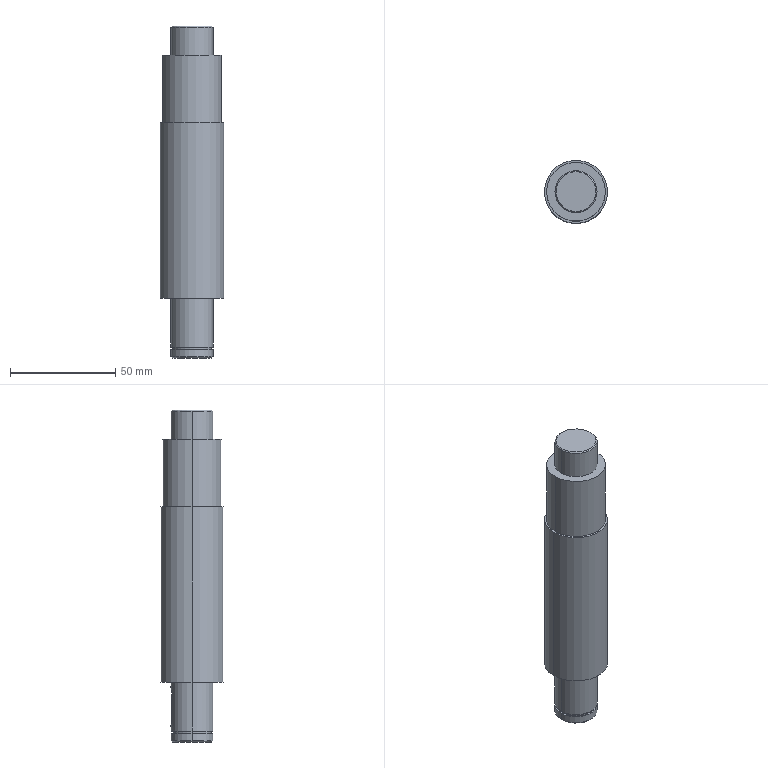Part | SolidWorks | features BaseBody 1 | 1 solid | 28 faces | box 30 x 30 x 157.8 mm | volume 91673 mm3 | cylinder 14 | plane 10 | cone 4 | commonest cylinder face diameters 20 x6 6 x2 18.35 x2 28 x2 30 x2
STEP:
#1=CARTESIAN_POINT('',(9.175,0.,5.2));
#2=VERTEX_POINT('',#1);
#3=CARTESIAN_POINT('',(-9.175,0.,5.2));
#4=VERTEX_POINT('',#3);
#5=CARTESIAN_POINT('',(0.,0.,5.2));
#6=DIRECTION('',(0.,0.,1.));
#7=DIRECTION('',(1.,0.,0.));
#8=AXIS2_PLACEMENT_3D('',#5,#6,#7);
#9=CIRCLE('',#8,9.175);
#10=EDGE_CURVE('',#2,#4,#9,.T.);
#11=ORIENTED_EDGE('',*,*,#10,.F.);
#12=CARTESIAN_POINT('',(9.175,0.,4.));
#13=VERTEX_POINT('',#12);
#14=CARTESIAN_POINT('',(9.175,0.,4.6));
#15=DIRECTION('',(0.,0.,-1.));
#16=VECTOR('',#15,1000.);
#17=LINE('',#14,#16);
#18=EDGE_CURVE('',#2,#13,#17,.T.);
#19=ORIENTED_EDGE('',*,*,#18,.T.);
#20=CARTESIAN_POINT('',(-9.175,0.,4.));
#21=VERTEX_POINT('',#20);
#22=CARTESIAN_POINT('',(0.,0.,4.));
#23=DIRECTION('',(0.,0.,1.));
#24=DIRECTION('',(1.,0.,0.));
#25=AXIS2_PLACEMENT_3D('',#22,#23,#24);
#26=CIRCLE('',#25,9.175);
#27=EDGE_CURVE('',#13,#21,#26,.T.);
#28=ORIENTED_EDGE('',*,*,#27,.T.);
#29=CARTESIAN_POINT('',(-9.175,0.,4.6));
#30=DIRECTION('',(0.,0.,-1.));
#31=VECTOR('',#30,1000.);
#32=LINE('',#29,#31);
#33=EDGE_CURVE('',#4,#21,#32,.T.);
#34=ORIENTED_EDGE('',*,*,#33,.F.);
#35=EDGE_LOOP('',(#11,#19,#28,#34));
#36=FACE_OUTER_BOUND('',#35,.T.);
#37=CARTESIAN_POINT('',(0.,0.,4.6));
#38=DIRECTION('',(0.,0.,-1.));
#39=DIRECTION('',(-1.,0.,0.));
#40=AXIS2_PLACEMENT_3D('',#37,#38,#39);
#41=CYLINDRICAL_SURFACE('',#40,9.175);
#42=ADVANCED_FACE('',(#36),#41,.T.);
#43=CARTESIAN_POINT('',(3.,9.539,10.789));
#44=VERTEX_POINT('',#43);
#45=CARTESIAN_POINT('',(3.,9.539,22.789));
#46=VERTEX_POINT('',#45);
#47=CARTESIAN_POINT('',(3.,9.539,0.));
#48=DIRECTION('',(0.,0.,1.));
#49=VECTOR('',#48,1000.);
#50=LINE('',#47,#49);
#51=EDGE_CURVE('',#44,#46,#50,.T.);
#52=ORIENTED_EDGE('',*,*,#51,.T.);
#53=CARTESIAN_POINT('',(-3.,9.539,22.789));
#54=VERTEX_POINT('',#53);
#55=CARTESIAN_POINT('',(3.,9.539,22.789));
#56=CARTESIAN_POINT('',(3.,9.539,22.988));
#57=CARTESIAN_POINT('',(2.98,9.546,23.184));
#58=CARTESIAN_POINT('',(2.904,9.569,23.569));
#59=CARTESIAN_POINT('',(2.845,9.587,23.76));
#60=CARTESIAN_POINT('',(2.695,9.63,24.122));
#61=CARTESIAN_POINT('',(2.602,9.656,24.294));
#62=CARTESIAN_POINT('',(2.385,9.712,24.619));
#63=CARTESIAN_POINT('',(2.259,9.742,24.772));
#64=CARTESIAN_POINT('',(1.847,9.832,25.185));
#65=CARTESIAN_POINT('',(1.515,9.891,25.408));
#66=CARTESIAN_POINT('',(0.9743,9.954,25.633));
#67=CARTESIAN_POINT('',(0.7844,9.971,25.691));
#68=CARTESIAN_POINT('',(0.396,9.994,25.769));
#69=CARTESIAN_POINT('',(0.1993,10.,25.789));
#70=CARTESIAN_POINT('',(-0.1994,10.,25.789));
#71=CARTESIAN_POINT('',(-0.3951,9.994,25.769));
#72=CARTESIAN_POINT('',(-0.7799,9.971,25.692));
#73=CARTESIAN_POINT('',(-0.971,9.954,25.634));
#74=CARTESIAN_POINT('',(-1.334,9.912,25.483));
#75=CARTESIAN_POINT('',(-1.505,9.887,25.391));
#76=CARTESIAN_POINT('',(-1.831,9.832,25.174));
#77=CARTESIAN_POINT('',(-1.984,9.802,25.048));
#78=CARTESIAN_POINT('',(-2.396,9.713,24.636));
#79=CARTESIAN_POINT('',(-2.619,9.652,24.303));
#80=CARTESIAN_POINT('',(-2.844,9.587,23.763));
#81=CARTESIAN_POINT('',(-2.902,9.57,23.573));
#82=CARTESIAN_POINT('',(-2.98,9.546,23.185));
#83=CARTESIAN_POINT('',(-3.,9.539,22.988));
#84=CARTESIAN_POINT('',(-3.,9.539,22.789));
#85=B_SPLINE_CURVE_WITH_KNOTS('',3,(#55,#56,#57,#58,#59,#60,#61,#62,#63,#64,#65,#66,#67,#68,#69,#70,#71,#72,#73,#74,#75,#76,#77,#78,#79,#80,#81,#82,#83,#84),.UNSPECIFIED.,.F.,.F.,(4,2,2,2,2,2,2,2,2,2,2,2,2,2,4),(0.,0.0005892,0.001178,0.001768,0.002357,0.003535,0.004125,0.004714,0.005303,0.005892,0.006482,0.007071,0.008249,0.008838,0.009428),.UNSPECIFIED.);
#86=EDGE_CURVE('',#46,#54,#85,.T.);
#87=ORIENTED_EDGE('',*,*,#86,.T.);
#88=CARTESIAN_POINT('',(-3.,9.539,10.789));
#89=VERTEX_POINT('',#88);
#90=CARTESIAN_POINT('',(-3.,9.539,0.));
#91=DIRECTION('',(0.,0.,-1.));
#92=VECTOR('',#91,1000.);
#93=LINE('',#90,#92);
#94=EDGE_CURVE('',#54,#89,#93,.T.);
#95=ORIENTED_EDGE('',*,*,#94,.T.);
#96=CARTESIAN_POINT('',(-3.,9.539,10.789));
#97=CARTESIAN_POINT('',(-3.,9.539,10.59));
#98=CARTESIAN_POINT('',(-2.98,9.546,10.394));
#99=CARTESIAN_POINT('',(-2.904,9.569,10.009));
#100=CARTESIAN_POINT('',(-2.845,9.587,9.818));
#101=CARTESIAN_POINT('',(-2.695,9.63,9.456));
#102=CARTESIAN_POINT('',(-2.602,9.656,9.284));
#103=CARTESIAN_POINT('',(-2.385,9.712,8.959));
#104=CARTESIAN_POINT('',(-2.259,9.742,8.806));
#105=CARTESIAN_POINT('',(-1.847,9.832,8.393));
#106=CARTESIAN_POINT('',(-1.515,9.891,8.17));
#107=CARTESIAN_POINT('',(-0.9743,9.954,7.945));
#108=CARTESIAN_POINT('',(-0.7844,9.971,7.887));
#109=CARTESIAN_POINT('',(-0.396,9.994,7.809));
#110=CARTESIAN_POINT('',(-0.1993,10.,7.789));
#111=CARTESIAN_POINT('',(0.1994,10.,7.789));
#112=CARTESIAN_POINT('',(0.3951,9.994,7.809));
#113=CARTESIAN_POINT('',(0.7799,9.971,7.886));
#114=CARTESIAN_POINT('',(0.971,9.954,7.944));
#115=CARTESIAN_POINT('',(1.334,9.912,8.095));
#116=CARTESIAN_POINT('',(1.505,9.887,8.187));
#117=CARTESIAN_POINT('',(1.831,9.832,8.404));
#118=CARTESIAN_POINT('',(1.984,9.802,8.53));
#119=CARTESIAN_POINT('',(2.396,9.713,8.942));
#120=CARTESIAN_POINT('',(2.619,9.652,9.275));
#121=CARTESIAN_POINT('',(2.844,9.587,9.815));
#122=CARTESIAN_POINT('',(2.902,9.57,10.005));
#123=CARTESIAN_POINT('',(2.98,9.546,10.393));
#124=CARTESIAN_POINT('',(3.,9.539,10.59));
#125=CARTESIAN_POINT('',(3.,9.539,10.789));
#126=B_SPLINE_CURVE_WITH_KNOTS('',3,(#96,#97,#98,#99,#100,#101,#102,#103,#104,#105,#106,#107,#108,#109,#110,#111,#112,#113,#114,#115,#116,#117,#118,#119,#120,#121,#122,#123,#124,#125),.UNSPECIFIED.,.F.,.F.,(4,2,2,2,2,2,2,2,2,2,2,2,2,2,4),(0.,0.0005892,0.001178,0.001768,0.002357,0.003535,0.004125,0.004714,0.005303,0.005892,0.006482,0.007071,0.008249,0.008838,0.009428),.UNSPECIFIED.);
#127=EDGE_CURVE('',#89,#44,#126,.T.);
#128=ORIENTED_EDGE('',*,*,#127,.T.);
#129=EDGE_LOOP('',(#52,#87,#95,#128));
#130=FACE_BOUND('',#129,.T.);
#131=CARTESIAN_POINT('',(10.,0.,28.378));
#132=VERTEX_POINT('',#131);
#133=CARTESIAN_POINT('',(-10.,0.,28.378));
#134=VERTEX_POINT('',#133);
#135=CARTESIAN_POINT('',(0.,0.,28.378));
#136=DIRECTION('',(0.,0.,1.));
#137=DIRECTION('',(-1.,0.,0.));
#138=AXIS2_PLACEMENT_3D('',#135,#136,#137);
#139=CIRCLE('',#138,10.);
#140=EDGE_CURVE('',#132,#134,#139,.T.);
#141=ORIENTED_EDGE('',*,*,#140,.F.);
#142=CARTESIAN_POINT('',(10.,0.,5.2));
#143=VERTEX_POINT('',#142);
#144=CARTESIAN_POINT('',(10.,0.,0.));
#145=DIRECTION('',(0.,0.,-1.));
#146=VECTOR('',#145,1000.);
#147=LINE('',#144,#146);
#148=EDGE_CURVE('',#132,#143,#147,.T.);
#149=ORIENTED_EDGE('',*,*,#148,.T.);
#150=CARTESIAN_POINT('',(-10.,0.,5.2));
#151=VERTEX_POINT('',#150);
#152=CARTESIAN_POINT('',(0.,0.,5.2));
#153=DIRECTION('',(0.,0.,1.));
#154=DIRECTION('',(-1.,0.,0.));
#155=AXIS2_PLACEMENT_3D('',#152,#153,#154);
#156=CIRCLE('',#155,10.);
#157=EDGE_CURVE('',#143,#151,#156,.T.);
#158=ORIENTED_EDGE('',*,*,#157,.T.);
#159=CARTESIAN_POINT('',(-10.,0.,0.));
#160=DIRECTION('',(0.,0.,-1.));
#161=VECTOR('',#160,1000.);
#162=LINE('',#159,#161);
#163=EDGE_CURVE('',#134,#151,#162,.T.);
#164=ORIENTED_EDGE('',*,*,#163,.F.);
#165=EDGE_LOOP('',(#141,#149,#158,#164));
#166=FACE_OUTER_BOUND('',#165,.T.);
#167=CARTESIAN_POINT('',(0.,0.,0.));
#168=DIRECTION('',(0.,0.,-1.));
#169=DIRECTION('',(-1.,0.,0.));
#170=AXIS2_PLACEMENT_3D('',#167,#168,#169);
#171=CYLINDRICAL_SURFACE('',#170,10.);
#172=ADVANCED_FACE('',(#130,#166),#171,.T.);
#173=CARTESIAN_POINT('',(-9.5,0.,157.8));
#174=VERTEX_POINT('',#173);
#175=CARTESIAN_POINT('',(9.5,0.,157.8));
#176=VERTEX_POINT('',#175);
#177=CARTESIAN_POINT('',(0.,0.,157.8));
#178=DIRECTION('',(0.,0.,-1.));
#179=DIRECTION('',(-1.,0.,0.));
#180=AXIS2_PLACEMENT_3D('',#177,#178,#179);
#181=CIRCLE('',#180,9.5);
#182=EDGE_CURVE('',#174,#176,#181,.T.);
#183=ORIENTED_EDGE('',*,*,#182,.T.);
#184=CARTESIAN_POINT('',(10.,0.,157.3));
#185=VERTEX_POINT('',#184);
#186=CARTESIAN_POINT('',(9.75,0.,157.55));
#187=DIRECTION('',(0.7071,0.,-0.7071));
#188=VECTOR('',#187,1000.);
#189=LINE('',#186,#188);
#190=EDGE_CURVE('',#176,#185,#189,.T.);
#191=ORIENTED_EDGE('',*,*,#190,.T.);
#192=CARTESIAN_POINT('',(-10.,0.,157.3));
#193=VERTEX_POINT('',#192);
#194=CARTESIAN_POINT('',(0.,0.,157.3));
#195=DIRECTION('',(0.,0.,1.));
#196=DIRECTION('',(-1.,0.,0.));
#197=AXIS2_PLACEMENT_3D('',#194,#195,#196);
#198=CIRCLE('',#197,10.);
#199=EDGE_CURVE('',#185,#193,#198,.T.);
#200=ORIENTED_EDGE('',*,*,#199,.T.);
#201=CARTESIAN_POINT('',(-9.75,0.,157.55));
#202=DIRECTION('',(-0.7071,0.,-0.7071));
#203=VECTOR('',#202,1000.);
#204=LINE('',#201,#203);
#205=EDGE_CURVE('',#174,#193,#204,.T.);
#206=ORIENTED_EDGE('',*,*,#205,.F.);
#207=EDGE_LOOP('',(#183,#191,#200,#206));
#208=FACE_OUTER_BOUND('',#207,.T.);
#209=CARTESIAN_POINT('',(0.,0.,157.55));
#210=DIRECTION('',(0.,0.,-1.));
#211=DIRECTION('',(-1.,0.,0.));
#212=AXIS2_PLACEMENT_3D('',#209,#210,#211);
#213=CONICAL_SURFACE('',#212,9.75,0.7854);
#214=ADVANCED_FACE('',(#208),#213,.T.);
#215=ORIENTED_EDGE('',*,*,#199,.F.);
#216=CARTESIAN_POINT('',(10.,0.,143.8));
#217=VERTEX_POINT('',#216);
#218=CARTESIAN_POINT('',(10.,0.,143.8));
#219=DIRECTION('',(0.,0.,-1.));
#220=VECTOR('',#219,1000.);
#221=LINE('',#218,#220);
#222=EDGE_CURVE('',#185,#217,#221,.T.);
#223=ORIENTED_EDGE('',*,*,#222,.T.);
#224=CARTESIAN_POINT('',(-10.,0.,143.8));
#225=VERTEX_POINT('',#224);
#226=CARTESIAN_POINT('',(0.,0.,143.8));
#227=DIRECTION('',(0.,0.,-1.));
#228=DIRECTION('',(-1.,0.,0.));
#229=AXIS2_PLACEMENT_3D('',#226,#227,#228);
#230=CIRCLE('',#229,10.);
#231=EDGE_CURVE('',#225,#217,#230,.T.);
#232=ORIENTED_EDGE('',*,*,#231,.F.);
#233=CARTESIAN_POINT('',(-10.,0.,143.8));
#234=DIRECTION('',(0.,0.,-1.));
#235=VECTOR('',#234,1000.);
#236=LINE('',#233,#235);
#237=EDGE_CURVE('',#193,#225,#236,.T.);
#238=ORIENTED_EDGE('',*,*,#237,.F.);
#239=EDGE_LOOP('',(#215,#223,#232,#238));
#240=FACE_OUTER_BOUND('',#239,.T.);
#241=CARTESIAN_POINT('',(0.,0.,143.8));
#242=DIRECTION('',(0.,0.,-1.));
#243=DIRECTION('',(-1.,0.,0.));
#244=AXIS2_PLACEMENT_3D('',#241,#242,#243);
#245=CYLINDRICAL_SURFACE('',#244,10.);
#246=ADVANCED_FACE('',(#240),#245,.T.);
#247=CARTESIAN_POINT('',(-9.5,0.,0.));
#248=VERTEX_POINT('',#247);
#249=CARTESIAN_POINT('',(9.5,0.,0.));
#250=VERTEX_POINT('',#249);
#251=CARTESIAN_POINT('',(0.,0.,0.));
#252=DIRECTION('',(0.,0.,1.));
#253=DIRECTION('',(-1.,0.,0.));
#254=AXIS2_PLACEMENT_3D('',#251,#252,#253);
#255=CIRCLE('',#254,9.5);
#256=EDGE_CURVE('',#248,#250,#255,.T.);
#257=ORIENTED_EDGE('',*,*,#256,.T.);
#258=CARTESIAN_POINT('',(10.,0.,0.5));
#259=VERTEX_POINT('',#258);
#260=CARTESIAN_POINT('',(9.75,0.,0.25));
#261=DIRECTION('',(0.7071,0.,0.7071));
#262=VECTOR('',#261,1000.);
#263=LINE('',#260,#262);
#264=EDGE_CURVE('',#250,#259,#263,.T.);
#265=ORIENTED_EDGE('',*,*,#264,.T.);
#266=CARTESIAN_POINT('',(-10.,0.,0.5));
#267=VERTEX_POINT('',#266);
#268=CARTESIAN_POINT('',(0.,0.,0.5));
#269=DIRECTION('',(0.,0.,-1.));
#270=DIRECTION('',(-1.,0.,0.));
#271=AXIS2_PLACEMENT_3D('',#268,#269,#270);
#272=CIRCLE('',#271,10.);
#273=EDGE_CURVE('',#259,#267,#272,.T.);
#274=ORIENTED_EDGE('',*,*,#273,.T.);
#275=CARTESIAN_POINT('',(-9.75,0.,0.25));
#276=DIRECTION('',(-0.7071,0.,0.7071));
#277=VECTOR('',#276,1000.);
#278=LINE('',#275,#277);
#279=EDGE_CURVE('',#248,#267,#278,.T.);
#280=ORIENTED_EDGE('',*,*,#279,.F.);
#281=EDGE_LOOP('',(#257,#265,#274,#280));
#282=FACE_OUTER_BOUND('',#281,.T.);
#283=CARTESIAN_POINT('',(0.,0.,0.25));
#284=DIRECTION('',(0.,0.,1.));
#285=DIRECTION('',(-1.,0.,0.));
#286=AXIS2_PLACEMENT_3D('',#283,#284,#285);
#287=CONICAL_SURFACE('',#286,9.75,0.7854);
#288=ADVANCED_FACE('',(#282),#287,.T.);
#289=CARTESIAN_POINT('',(-10.,0.,4.));
#290=VERTEX_POINT('',#289);
#291=CARTESIAN_POINT('',(10.,0.,4.));
#292=VERTEX_POINT('',#291);
#293=CARTESIAN_POINT('',(0.,0.,4.));
#294=DIRECTION('',(0.,0.,-1.));
#295=DIRECTION('',(-1.,0.,0.));
#296=AXIS2_PLACEMENT_3D('',#293,#294,#295);
#297=CIRCLE('',#296,10.);
#298=EDGE_CURVE('',#290,#292,#297,.T.);
#299=ORIENTED_EDGE('',*,*,#298,.T.);
#300=CARTESIAN_POINT('',(10.,0.,0.));
#301=DIRECTION('',(0.,0.,-1.));
#302=VECTOR('',#301,1000.);
#303=LINE('',#300,#302);
#304=EDGE_CURVE('',#292,#259,#303,.T.);
#305=ORIENTED_EDGE('',*,*,#304,.T.);
#306=CARTESIAN_POINT('',(0.,0.,0.5));
#307=DIRECTION('',(0.,0.,-1.));
#308=DIRECTION('',(-1.,0.,0.));
#309=AXIS2_PLACEMENT_3D('',#306,#307,#308);
#310=CIRCLE('',#309,10.);
#311=EDGE_CURVE('',#267,#259,#310,.T.);
#312=ORIENTED_EDGE('',*,*,#311,.F.);
#313=CARTESIAN_POINT('',(-10.,0.,0.));
#314=DIRECTION('',(0.,0.,-1.));
#315=VECTOR('',#314,1000.);
#316=LINE('',#313,#315);
#317=EDGE_CURVE('',#290,#267,#316,.T.);
#318=ORIENTED_EDGE('',*,*,#317,.F.);
#319=EDGE_LOOP('',(#299,#305,#312,#318));
#320=FACE_OUTER_BOUND('',#319,.T.);
#321=CARTESIAN_POINT('',(0.,0.,0.));
#322=DIRECTION('',(0.,0.,-1.));
#323=DIRECTION('',(-1.,0.,0.));
#324=AXIS2_PLACEMENT_3D('',#321,#322,#323);
#325=CYLINDRICAL_SURFACE('',#324,10.);
#326=ADVANCED_FACE('',(#320),#325,.T.);
#327=CARTESIAN_POINT('',(14.,0.,143.8));
#328=VERTEX_POINT('',#327);
#329=CARTESIAN_POINT('',(-14.,0.,143.8));
#330=VERTEX_POINT('',#329);
#331=CARTESIAN_POINT('',(0.,0.,143.8));
#332=DIRECTION('',(0.,0.,1.));
#333=DIRECTION('',(-1.,0.,0.));
#334=AXIS2_PLACEMENT_3D('',#331,#332,#333);
#335=CIRCLE('',#334,14.);
#336=EDGE_CURVE('',#328,#330,#335,.T.);
#337=ORIENTED_EDGE('',*,*,#336,.F.);
#338=CARTESIAN_POINT('',(14.,0.,111.8));
#339=VERTEX_POINT('',#338);
#340=CARTESIAN_POINT('',(14.,0.,111.8));
#341=DIRECTION('',(0.,0.,-1.));
#342=VECTOR('',#341,1000.);
#343=LINE('',#340,#342);
#344=EDGE_CURVE('',#328,#339,#343,.T.);
#345=ORIENTED_EDGE('',*,*,#344,.T.);
#346=CARTESIAN_POINT('',(-14.,0.,111.8));
#347=VERTEX_POINT('',#346);
#348=CARTESIAN_POINT('',(0.,0.,111.8));
#349=DIRECTION('',(0.,0.,-1.));
#350=DIRECTION('',(-1.,0.,0.));
#351=AXIS2_PLACEMENT_3D('',#348,#349,#350);
#352=CIRCLE('',#351,14.);
#353=EDGE_CURVE('',#347,#339,#352,.T.);
#354=ORIENTED_EDGE('',*,*,#353,.F.);
#355=CARTESIAN_POINT('',(-14.,0.,111.8));
#356=DIRECTION('',(0.,0.,-1.));
#357=VECTOR('',#356,1000.);
#358=LINE('',#355,#357);
#359=EDGE_CURVE('',#330,#347,#358,.T.);
#360=ORIENTED_EDGE('',*,*,#359,.F.);
#361=EDGE_LOOP('',(#337,#345,#354,#360));
#362=FACE_OUTER_BOUND('',#361,.T.);
#363=CARTESIAN_POINT('',(0.,0.,111.8));
#364=DIRECTION('',(0.,0.,-1.));
#365=DIRECTION('',(-1.,0.,0.));
#366=AXIS2_PLACEMENT_3D('',#363,#364,#365);
#367=CYLINDRICAL_SURFACE('',#366,14.);
#368=ADVANCED_FACE('',(#362),#367,.T.);
#369=CARTESIAN_POINT('',(15.,0.,111.8));
#370=VERTEX_POINT('',#369);
#371=CARTESIAN_POINT('',(-15.,0.,111.8));
#372=VERTEX_POINT('',#371);
#373=CARTESIAN_POINT('',(0.,0.,111.8));
#374=DIRECTION('',(0.,0.,1.));
#375=DIRECTION('',(-1.,0.,0.));
#376=AXIS2_PLACEMENT_3D('',#373,#374,#375);
#377=CIRCLE('',#376,15.);
#378=EDGE_CURVE('',#370,#372,#377,.T.);
#379=ORIENTED_EDGE('',*,*,#378,.F.);
#380=CARTESIAN_POINT('',(15.,0.,28.378));
#381=VERTEX_POINT('',#380);
#382=CARTESIAN_POINT('',(15.,0.,28.378));
#383=DIRECTION('',(0.,0.,-1.));
#384=VECTOR('',#383,1000.);
#385=LINE('',#382,#384);
#386=EDGE_CURVE('',#370,#381,#385,.T.);
#387=ORIENTED_EDGE('',*,*,#386,.T.);
#388=CARTESIAN_POINT('',(-15.,0.,28.378));
#389=VERTEX_POINT('',#388);
#390=CARTESIAN_POINT('',(0.,0.,28.378));
#391=DIRECTION('',(0.,0.,-1.));
#392=DIRECTION('',(-1.,0.,0.));
#393=AXIS2_PLACEMENT_3D('',#390,#391,#392);
#394=CIRCLE('',#393,15.);
#395=EDGE_CURVE('',#389,#381,#394,.T.);
#396=ORIENTED_EDGE('',*,*,#395,.F.);
#397=CARTESIAN_POINT('',(-15.,0.,28.378));
#398=DIRECTION('',(0.,0.,-1.));
#399=VECTOR('',#398,1000.);
#400=LINE('',#397,#399);
#401=EDGE_CURVE('',#372,#389,#400,.T.);
#402=ORIENTED_EDGE('',*,*,#401,.F.);
#403=EDGE_LOOP('',(#379,#387,#396,#402));
#404=FACE_OUTER_BOUND('',#403,.T.);
#405=CARTESIAN_POINT('',(0.,0.,28.378));
#406=DIRECTION('',(0.,0.,-1.));
#407=DIRECTION('',(-1.,0.,0.));
#408=AXIS2_PLACEMENT_3D('',#405,#406,#407);
#409=CYLINDRICAL_SURFACE('',#408,15.);
#410=ADVANCED_FACE('',(#404),#409,.T.);
#411=CARTESIAN_POINT('',(0.,0.,4.));
#412=DIRECTION('',(0.,0.,1.));
#413=DIRECTION('',(1.,0.,0.));
#414=AXIS2_PLACEMENT_3D('',#411,#412,#413);
#415=CIRCLE('',#414,9.175);
#416=EDGE_CURVE('',#21,#13,#415,.T.);
#417=ORIENTED_EDGE('',*,*,#416,.F.);
#418=ORIENTED_EDGE('',*,*,#27,.F.);
#419=EDGE_LOOP('',(#417,#418));
#420=FACE_BOUND('',#419,.T.);
#421=ORIENTED_EDGE('',*,*,#298,.F.);
#422=CARTESIAN_POINT('',(0.,0.,4.));
#423=DIRECTION('',(0.,0.,-1.));
#424=DIRECTION('',(-1.,0.,0.));
#425=AXIS2_PLACEMENT_3D('',#422,#423,#424);
#426=CIRCLE('',#425,10.);
#427=EDGE_CURVE('',#292,#290,#426,.T.);
#428=ORIENTED_EDGE('',*,*,#427,.F.);
#429=EDGE_LOOP('',(#421,#428));
#430=FACE_OUTER_BOUND('',#429,.T.);
#431=CARTESIAN_POINT('',(-14.411,0.,4.));
#432=DIRECTION('',(0.,0.,-1.));
#433=DIRECTION('',(0.,-1.,0.));
#434=AXIS2_PLACEMENT_3D('',#431,#432,#433);
#435=PLANE('',#434);
#436=ADVANCED_FACE('',(#420,#430),#435,.F.);
#437=CARTESIAN_POINT('',(0.,0.,5.2));
#438=DIRECTION('',(0.,0.,1.));
#439=DIRECTION('',(1.,0.,0.));
#440=AXIS2_PLACEMENT_3D('',#437,#438,#439);
#441=CIRCLE('',#440,9.175);
#442=EDGE_CURVE('',#4,#2,#441,.T.);
#443=ORIENTED_EDGE('',*,*,#442,.T.);
#444=ORIENTED_EDGE('',*,*,#10,.T.);
#445=EDGE_LOOP('',(#443,#444));
#446=FACE_BOUND('',#445,.T.);
#447=CARTESIAN_POINT('',(0.,0.,5.2));
#448=DIRECTION('',(0.,0.,1.));
#449=DIRECTION('',(-1.,0.,0.));
#450=AXIS2_PLACEMENT_3D('',#447,#448,#449);
#451=CIRCLE('',#450,10.);
#452=EDGE_CURVE('',#151,#143,#451,.T.);
#453=ORIENTED_EDGE('',*,*,#452,.F.);
#454=ORIENTED_EDGE('',*,*,#157,.F.);
#455=EDGE_LOOP('',(#453,#454));
#456=FACE_OUTER_BOUND('',#455,.T.);
#457=CARTESIAN_POINT('',(-9.175,0.,5.2));
#458=DIRECTION('',(0.,0.,1.));
#459=DIRECTION('',(1.,0.,0.));
#460=AXIS2_PLACEMENT_3D('',#457,#458,#459);
#461=PLANE('',#460);
#462=ADVANCED_FACE('',(#446,#456),#461,.F.);
#463=ORIENTED_EDGE('',*,*,#182,.F.);
#464=CARTESIAN_POINT('',(0.,0.,157.8));
#465=DIRECTION('',(0.,0.,-1.));
#466=DIRECTION('',(-1.,0.,0.));
#467=AXIS2_PLACEMENT_3D('',#464,#465,#466);
#468=CIRCLE('',#467,9.5);
#469=EDGE_CURVE('',#176,#174,#468,.T.);
#470=ORIENTED_EDGE('',*,*,#469,.F.);
#471=EDGE_LOOP('',(#463,#470));
#472=FACE_OUTER_BOUND('',#471,.T.);
#473=CARTESIAN_POINT('',(0.,0.,157.8));
#474=DIRECTION('',(0.,0.,1.));
#475=DIRECTION('',(1.,0.,0.));
#476=AXIS2_PLACEMENT_3D('',#473,#474,#475);
#477=PLANE('',#476);
#478=ADVANCED_FACE('',(#472),#477,.T.);
#479=ORIENTED_EDGE('',*,*,#256,.F.);
#480=CARTESIAN_POINT('',(0.,0.,0.));
#481=DIRECTION('',(0.,0.,1.));
#482=DIRECTION('',(-1.,0.,0.));
#483=AXIS2_PLACEMENT_3D('',#480,#481,#482);
#484=CIRCLE('',#483,9.5);
#485=EDGE_CURVE('',#250,#248,#484,.T.);
#486=ORIENTED_EDGE('',*,*,#485,.F.);
#487=EDGE_LOOP('',(#479,#486));
#488=FACE_OUTER_BOUND('',#487,.T.);
#489=CARTESIAN_POINT('',(0.,0.,0.));
#490=DIRECTION('',(0.,0.,1.));
#491=DIRECTION('',(1.,0.,0.));
#492=AXIS2_PLACEMENT_3D('',#489,#490,#491);
#493=PLANE('',#492);
#494=ADVANCED_FACE('',(#488),#493,.F.);
#495=ORIENTED_EDGE('',*,*,#94,.F.);
#496=CARTESIAN_POINT('',(-3.,7.5,22.789));
#497=VERTEX_POINT('',#496);
#498=CARTESIAN_POINT('',(-3.,10.,22.789));
#499=DIRECTION('',(0.,-1.,0.));
#500=VECTOR('',#499,1000.);
#501=LINE('',#498,#500);
#502=EDGE_CURVE('',#54,#497,#501,.T.);
#503=ORIENTED_EDGE('',*,*,#502,.T.);
#504=CARTESIAN_POINT('',(-3.,7.5,10.789));
#505=VERTEX_POINT('',#504);
#506=CARTESIAN_POINT('',(-3.,7.5,10.789));
#507=DIRECTION('',(0.,0.,-1.));
#508=VECTOR('',#507,1000.);
#509=LINE('',#506,#508);
#510=EDGE_CURVE('',#497,#505,#509,.T.);
#511=ORIENTED_EDGE('',*,*,#510,.T.);
#512=CARTESIAN_POINT('',(-3.,10.,10.789));
#513=DIRECTION('',(0.,-1.,0.));
#514=VECTOR('',#513,1000.);
#515=LINE('',#512,#514);
#516=EDGE_CURVE('',#89,#505,#515,.T.);
#517=ORIENTED_EDGE('',*,*,#516,.F.);
#518=EDGE_LOOP('',(#495,#503,#511,#517));
#519=FACE_OUTER_BOUND('',#518,.T.);
#520=CARTESIAN_POINT('',(-3.,10.,22.789));
#521=DIRECTION('',(-1.,0.,0.));
#522=DIRECTION('',(0.,0.,1.));
#523=AXIS2_PLACEMENT_3D('',#520,#521,#522);
#524=PLANE('',#523);
#525=ADVANCED_FACE('',(#519),#524,.F.);
#526=ORIENTED_EDGE('',*,*,#127,.F.);
#527=ORIENTED_EDGE('',*,*,#516,.T.);
#528=CARTESIAN_POINT('',(3.,7.5,10.789));
#529=VERTEX_POINT('',#528);
#530=CARTESIAN_POINT('',(0.,7.5,10.789));
#531=DIRECTION('',(0.,-1.,0.));
#532=DIRECTION('',(1.,0.,0.));
#533=AXIS2_PLACEMENT_3D('',#530,#531,#532);
#534=CIRCLE('',#533,3.);
#535=EDGE_CURVE('',#505,#529,#534,.T.);
#536=ORIENTED_EDGE('',*,*,#535,.T.);
#537=CARTESIAN_POINT('',(3.,10.,10.789));
#538=DIRECTION('',(0.,-1.,0.));
#539=VECTOR('',#538,1000.);
#540=LINE('',#537,#539);
#541=EDGE_CURVE('',#44,#529,#540,.T.);
#542=ORIENTED_EDGE('',*,*,#541,.F.);
#543=EDGE_LOOP('',(#526,#527,#536,#542));
#544=FACE_OUTER_BOUND('',#543,.T.);
#545=CARTESIAN_POINT('',(0.,10.,10.789));
#546=DIRECTION('',(0.,1.,0.));
#547=DIRECTION('',(1.,0.,0.));
#548=AXIS2_PLACEMENT_3D('',#545,#546,#547);
#549=CYLINDRICAL_SURFACE('',#548,3.);
#550=ADVANCED_FACE('',(#544),#549,.F.);
#551=ORIENTED_EDGE('',*,*,#51,.F.);
#552=ORIENTED_EDGE('',*,*,#541,.T.);
#553=CARTESIAN_POINT('',(3.,7.5,22.789));
#554=VERTEX_POINT('',#553);
#555=CARTESIAN_POINT('',(3.,7.5,22.789));
#556=DIRECTION('',(0.,0.,1.));
#557=VECTOR('',#556,1000.);
#558=LINE('',#555,#557);
#559=EDGE_CURVE('',#529,#554,#558,.T.);
#560=ORIENTED_EDGE('',*,*,#559,.T.);
#561=CARTESIAN_POINT('',(3.,10.,22.789));
#562=DIRECTION('',(0.,-1.,0.));
#563=VECTOR('',#562,1000.);
#564=LINE('',#561,#563);
#565=EDGE_CURVE('',#46,#554,#564,.T.);
#566=ORIENTED_EDGE('',*,*,#565,.F.);
#567=EDGE_LOOP('',(#551,#552,#560,#566));
#568=FACE_OUTER_BOUND('',#567,.T.);
#569=CARTESIAN_POINT('',(3.,10.,10.789));
#570=DIRECTION('',(1.,0.,0.));
#571=DIRECTION('',(0.,0.,-1.));
#572=AXIS2_PLACEMENT_3D('',#569,#570,#571);
#573=PLANE('',#572);
#574=ADVANCED_FACE('',(#568),#573,.F.);
#575=ORIENTED_EDGE('',*,*,#502,.F.);
#576=ORIENTED_EDGE('',*,*,#86,.F.);
#577=ORIENTED_EDGE('',*,*,#565,.T.);
#578=CARTESIAN_POINT('',(0.,7.5,22.789));
#579=DIRECTION('',(0.,-1.,0.));
#580=DIRECTION('',(-1.,0.,0.));
#581=AXIS2_PLACEMENT_3D('',#578,#579,#580);
#582=CIRCLE('',#581,3.);
#583=EDGE_CURVE('',#554,#497,#582,.T.);
#584=ORIENTED_EDGE('',*,*,#583,.T.);
#585=EDGE_LOOP('',(#575,#576,#577,#584));
#586=FACE_OUTER_BOUND('',#585,.T.);
#587=CARTESIAN_POINT('',(0.,10.,22.789));
#588=DIRECTION('',(0.,1.,0.));
#589=DIRECTION('',(-1.,0.,0.));
#590=AXIS2_PLACEMENT_3D('',#587,#588,#589);
#591=CYLINDRICAL_SURFACE('',#590,3.);
#592=ADVANCED_FACE('',(#586),#591,.F.);
#593=ORIENTED_EDGE('',*,*,#583,.F.);
#594=ORIENTED_EDGE('',*,*,#559,.F.);
#595=ORIENTED_EDGE('',*,*,#535,.F.);
#596=ORIENTED_EDGE('',*,*,#510,.F.);
#597=EDGE_LOOP('',(#593,#594,#595,#596));
#598=FACE_OUTER_BOUND('',#597,.T.);
#599=CARTESIAN_POINT('',(0.,7.5,23.822));
#600=DIRECTION('',(0.,1.,0.));
#601=DIRECTION('',(1.,0.,0.));
#602=AXIS2_PLACEMENT_3D('',#599,#600,#601);
#603=PLANE('',#602);
#604=ADVANCED_FACE('',(#598),#603,.T.);
#605=ORIENTED_EDGE('',*,*,#231,.T.);
#606=CARTESIAN_POINT('',(0.,0.,143.8));
#607=DIRECTION('',(0.,0.,-1.));
#608=DIRECTION('',(-1.,0.,0.));
#609=AXIS2_PLACEMENT_3D('',#606,#607,#608);
#610=CIRCLE('',#609,10.);
#611=EDGE_CURVE('',#217,#225,#610,.T.);
#612=ORIENTED_EDGE('',*,*,#611,.T.);
#613=EDGE_LOOP('',(#605,#612));
#614=FACE_BOUND('',#613,.T.);
#615=CARTESIAN_POINT('',(0.,0.,143.8));
#616=DIRECTION('',(0.,0.,1.));
#617=DIRECTION('',(-1.,0.,0.));
#618=AXIS2_PLACEMENT_3D('',#615,#616,#617);
#619=CIRCLE('',#618,14.);
#620=EDGE_CURVE('',#330,#328,#619,.T.);
#621=ORIENTED_EDGE('',*,*,#620,.T.);
#622=ORIENTED_EDGE('',*,*,#336,.T.);
#623=EDGE_LOOP('',(#621,#622));
#624=FACE_OUTER_BOUND('',#623,.T.);
#625=CARTESIAN_POINT('',(0.,0.,143.8));
#626=DIRECTION('',(0.,0.,1.));
#627=DIRECTION('',(1.,0.,0.));
#628=AXIS2_PLACEMENT_3D('',#625,#626,#627);
#629=PLANE('',#628);
#630=ADVANCED_FACE('',(#614,#624),#629,.T.);
#631=CARTESIAN_POINT('',(0.,0.,28.378));
#632=DIRECTION('',(0.,0.,1.));
#633=DIRECTION('',(-1.,0.,0.));
#634=AXIS2_PLACEMENT_3D('',#631,#632,#633);
#635=CIRCLE('',#634,10.);
#636=EDGE_CURVE('',#134,#132,#635,.T.);
#637=ORIENTED_EDGE('',*,*,#636,.T.);
#638=ORIENTED_EDGE('',*,*,#140,.T.);
#639=EDGE_LOOP('',(#637,#638));
#640=FACE_BOUND('',#639,.T.);
#641=ORIENTED_EDGE('',*,*,#395,.T.);
#642=CARTESIAN_POINT('',(0.,0.,28.378));
#643=DIRECTION('',(0.,0.,-1.));
#644=DIRECTION('',(-1.,0.,0.));
#645=AXIS2_PLACEMENT_3D('',#642,#643,#644);
#646=CIRCLE('',#645,15.);
#647=EDGE_CURVE('',#381,#389,#646,.T.);
#648=ORIENTED_EDGE('',*,*,#647,.T.);
#649=EDGE_LOOP('',(#641,#648));
#650=FACE_OUTER_BOUND('',#649,.T.);
#651=CARTESIAN_POINT('',(0.,0.,28.378));
#652=DIRECTION('',(0.,0.,1.));
#653=DIRECTION('',(1.,0.,0.));
#654=AXIS2_PLACEMENT_3D('',#651,#652,#653);
#655=PLANE('',#654);
#656=ADVANCED_FACE('',(#640,#650),#655,.F.);
#657=ORIENTED_EDGE('',*,*,#353,.T.);
#658=CARTESIAN_POINT('',(0.,0.,111.8));
#659=DIRECTION('',(0.,0.,-1.));
#660=DIRECTION('',(-1.,0.,0.));
#661=AXIS2_PLACEMENT_3D('',#658,#659,#660);
#662=CIRCLE('',#661,14.);
#663=EDGE_CURVE('',#339,#347,#662,.T.);
#664=ORIENTED_EDGE('',*,*,#663,.T.);
#665=EDGE_LOOP('',(#657,#664));
#666=FACE_BOUND('',#665,.T.);
#667=CARTESIAN_POINT('',(0.,0.,111.8));
#668=DIRECTION('',(0.,0.,1.));
#669=DIRECTION('',(-1.,0.,0.));
#670=AXIS2_PLACEMENT_3D('',#667,#668,#669);
#671=CIRCLE('',#670,15.);
#672=EDGE_CURVE('',#372,#370,#671,.T.);
#673=ORIENTED_EDGE('',*,*,#672,.T.);
#674=ORIENTED_EDGE('',*,*,#378,.T.);
#675=EDGE_LOOP('',(#673,#674));
#676=FACE_OUTER_BOUND('',#675,.T.);
#677=CARTESIAN_POINT('',(0.,0.,111.8));
#678=DIRECTION('',(0.,0.,1.));
#679=DIRECTION('',(1.,0.,0.));
#680=AXIS2_PLACEMENT_3D('',#677,#678,#679);
#681=PLANE('',#680);
#682=ADVANCED_FACE('',(#666,#676),#681,.T.);
#683=ORIENTED_EDGE('',*,*,#386,.F.);
#684=ORIENTED_EDGE('',*,*,#672,.F.);
#685=ORIENTED_EDGE('',*,*,#401,.T.);
#686=ORIENTED_EDGE('',*,*,#647,.F.);
#687=EDGE_LOOP('',(#683,#684,#685,#686));
#688=FACE_OUTER_BOUND('',#687,.T.);
#689=CARTESIAN_POINT('',(0.,0.,28.378));
#690=DIRECTION('',(0.,0.,-1.));
#691=DIRECTION('',(-1.,0.,0.));
#692=AXIS2_PLACEMENT_3D('',#689,#690,#691);
#693=CYLINDRICAL_SURFACE('',#692,15.);
#694=ADVANCED_FACE('',(#688),#693,.T.);
#695=ORIENTED_EDGE('',*,*,#344,.F.);
#696=ORIENTED_EDGE('',*,*,#620,.F.);
#697=ORIENTED_EDGE('',*,*,#359,.T.);
#698=ORIENTED_EDGE('',*,*,#663,.F.);
#699=EDGE_LOOP('',(#695,#696,#697,#698));
#700=FACE_OUTER_BOUND('',#699,.T.);
#701=CARTESIAN_POINT('',(0.,0.,111.8));
#702=DIRECTION('',(0.,0.,-1.));
#703=DIRECTION('',(-1.,0.,0.));
#704=AXIS2_PLACEMENT_3D('',#701,#702,#703);
#705=CYLINDRICAL_SURFACE('',#704,14.);
#706=ADVANCED_FACE('',(#700),#705,.T.);
#707=ORIENTED_EDGE('',*,*,#304,.F.);
#708=ORIENTED_EDGE('',*,*,#427,.T.);
#709=ORIENTED_EDGE('',*,*,#317,.T.);
#710=ORIENTED_EDGE('',*,*,#273,.F.);
#711=EDGE_LOOP('',(#707,#708,#709,#710));
#712=FACE_OUTER_BOUND('',#711,.T.);
#713=CARTESIAN_POINT('',(0.,0.,0.));
#714=DIRECTION('',(0.,0.,-1.));
#715=DIRECTION('',(-1.,0.,0.));
#716=AXIS2_PLACEMENT_3D('',#713,#714,#715);
#717=CYLINDRICAL_SURFACE('',#716,10.);
#718=ADVANCED_FACE('',(#712),#717,.T.);
#719=ORIENTED_EDGE('',*,*,#264,.F.);
#720=ORIENTED_EDGE('',*,*,#485,.T.);
#721=ORIENTED_EDGE('',*,*,#279,.T.);
#722=ORIENTED_EDGE('',*,*,#311,.T.);
#723=EDGE_LOOP('',(#719,#720,#721,#722));
#724=FACE_OUTER_BOUND('',#723,.T.);
#725=CARTESIAN_POINT('',(0.,0.,0.25));
#726=DIRECTION('',(0.,0.,1.));
#727=DIRECTION('',(-1.,0.,0.));
#728=AXIS2_PLACEMENT_3D('',#725,#726,#727);
#729=CONICAL_SURFACE('',#728,9.75,0.7854);
#730=ADVANCED_FACE('',(#724),#729,.T.);
#731=ORIENTED_EDGE('',*,*,#222,.F.);
#732=CARTESIAN_POINT('',(0.,0.,157.3));
#733=DIRECTION('',(0.,0.,1.));
#734=DIRECTION('',(-1.,0.,0.));
#735=AXIS2_PLACEMENT_3D('',#732,#733,#734);
#736=CIRCLE('',#735,10.);
#737=EDGE_CURVE('',#193,#185,#736,.T.);
#738=ORIENTED_EDGE('',*,*,#737,.F.);
#739=ORIENTED_EDGE('',*,*,#237,.T.);
#740=ORIENTED_EDGE('',*,*,#611,.F.);
#741=EDGE_LOOP('',(#731,#738,#739,#740));
#742=FACE_OUTER_BOUND('',#741,.T.);
#743=CARTESIAN_POINT('',(0.,0.,143.8));
#744=DIRECTION('',(0.,0.,-1.));
#745=DIRECTION('',(-1.,0.,0.));
#746=AXIS2_PLACEMENT_3D('',#743,#744,#745);
#747=CYLINDRICAL_SURFACE('',#746,10.);
#748=ADVANCED_FACE('',(#742),#747,.T.);
#749=ORIENTED_EDGE('',*,*,#190,.F.);
#750=ORIENTED_EDGE('',*,*,#469,.T.);
#751=ORIENTED_EDGE('',*,*,#205,.T.);
#752=ORIENTED_EDGE('',*,*,#737,.T.);
#753=EDGE_LOOP('',(#749,#750,#751,#752));
#754=FACE_OUTER_BOUND('',#753,.T.);
#755=CARTESIAN_POINT('',(0.,0.,157.55));
#756=DIRECTION('',(0.,0.,-1.));
#757=DIRECTION('',(-1.,0.,0.));
#758=AXIS2_PLACEMENT_3D('',#755,#756,#757);
#759=CONICAL_SURFACE('',#758,9.75,0.7854);
#760=ADVANCED_FACE('',(#754),#759,.T.);
#761=ORIENTED_EDGE('',*,*,#148,.F.);
#762=ORIENTED_EDGE('',*,*,#636,.F.);
#763=ORIENTED_EDGE('',*,*,#163,.T.);
#764=ORIENTED_EDGE('',*,*,#452,.T.);
#765=EDGE_LOOP('',(#761,#762,#763,#764));
#766=FACE_OUTER_BOUND('',#765,.T.);
#767=CARTESIAN_POINT('',(0.,0.,0.));
#768=DIRECTION('',(0.,0.,-1.));
#769=DIRECTION('',(-1.,0.,0.));
#770=AXIS2_PLACEMENT_3D('',#767,#768,#769);
#771=CYLINDRICAL_SURFACE('',#770,10.);
#772=ADVANCED_FACE('',(#766),#771,.T.);
#773=ORIENTED_EDGE('',*,*,#18,.F.);
#774=ORIENTED_EDGE('',*,*,#442,.F.);
#775=ORIENTED_EDGE('',*,*,#33,.T.);
#776=ORIENTED_EDGE('',*,*,#416,.T.);
#777=EDGE_LOOP('',(#773,#774,#775,#776));
#778=FACE_OUTER_BOUND('',#777,.T.);
#779=CARTESIAN_POINT('',(0.,0.,4.6));
#780=DIRECTION('',(0.,0.,-1.));
#781=DIRECTION('',(-1.,0.,0.));
#782=AXIS2_PLACEMENT_3D('',#779,#780,#781);
#783=CYLINDRICAL_SURFACE('',#782,9.175);
#784=ADVANCED_FACE('',(#778),#783,.T.);
#785=CLOSED_SHELL('',(#42,#172,#214,#246,#288,#326,#368,#410,#436,#462,#478,#494,#525,#550,#574,#592,#604,#630,#656,#682,#694,#706,#718,#730,#748,#760,#772,#784));
#786=MANIFOLD_SOLID_BREP('',#785);
#787=CARTESIAN_POINT('',(0.,0.,0.));
#788=DIRECTION('',(0.,0.,1.));
#789=DIRECTION('',(1.,0.,0.));
#790=AXIS2_PLACEMENT_3D('',#787,#788,#789);
#791=(LENGTH_UNIT()NAMED_UNIT(*)SI_UNIT(.MILLI.,.METRE.));
#792=UNCERTAINTY_MEASURE_WITH_UNIT(LENGTH_MEASURE(0.00001),#791,'','');
#793=(NAMED_UNIT(*)PLANE_ANGLE_UNIT()SI_UNIT($,.RADIAN.));
#794=(NAMED_UNIT(*)SI_UNIT($,.STERADIAN.)SOLID_ANGLE_UNIT());
#795=(GEOMETRIC_REPRESENTATION_CONTEXT(3)GLOBAL_UNCERTAINTY_ASSIGNED_CONTEXT((#792))GLOBAL_UNIT_ASSIGNED_CONTEXT((#791,#793,#794))REPRESENTATION_CONTEXT('',''));
#796=ADVANCED_BREP_SHAPE_REPRESENTATION('',(#786,#790),#795);